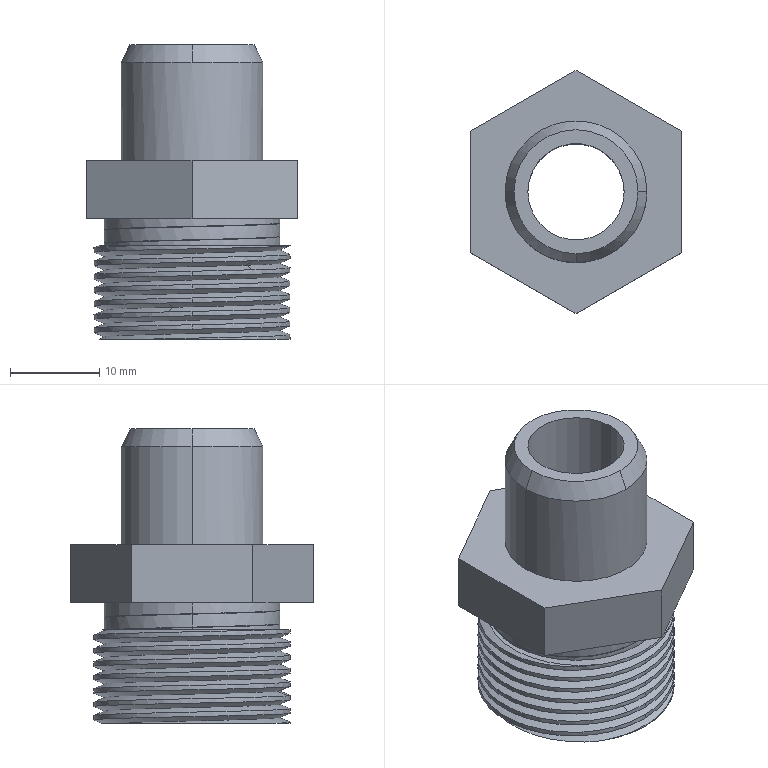Part | SolidWorks | features BaseBody 1 | 1 solid | 45 faces | box 23.6 x 27.251 x 33 mm | volume 7269 mm3 | cylinder 24 | plane 12 | spline 6 | cone 3 | commonest cylinder face diameters 22 x14 19.7 x6 10.8 x2 15.9 x2